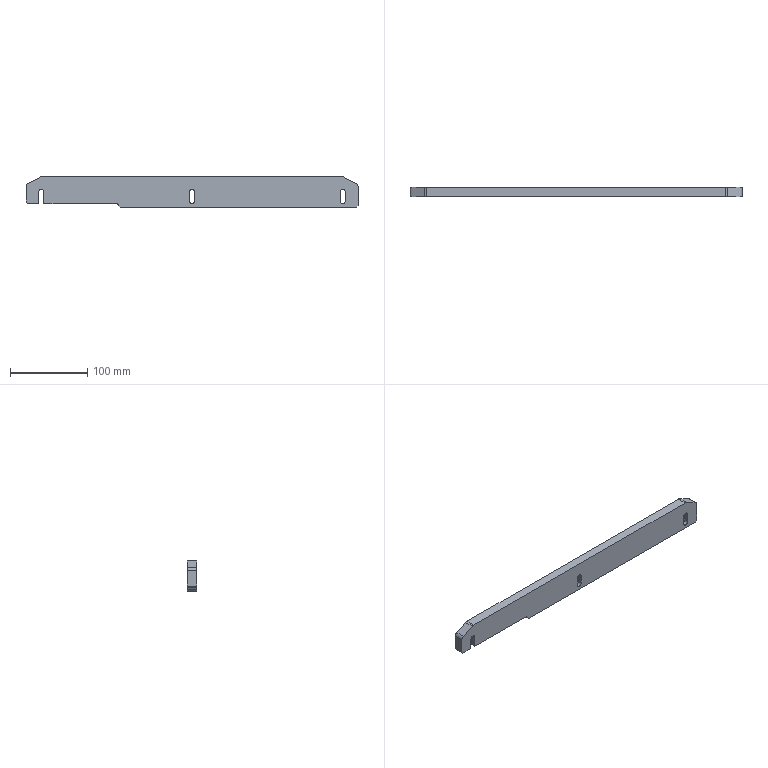Part | 1 solid | 43 faces | box 430.5 x 12 x 40 mm | volume 190634 mm3 | plane 28 | cylinder 15 | commonest cylinder face diameters 6.6 x5 11 x5 10 x4 6 x1
STEP:
#1=CARTESIAN_POINT('',(-95.25,-6.,-18.));
#2=VERTEX_POINT('',#1);
#3=CARTESIAN_POINT('',(-93.25,-6.,-20.));
#4=VERTEX_POINT('',#3);
#5=CARTESIAN_POINT('',(-93.25,-6.,-20.));
#6=DIRECTION('',(0.7071,0.,-0.7071));
#7=VECTOR('',#6,1000.);
#8=LINE('',#5,#7);
#9=EDGE_CURVE('',#2,#4,#8,.T.);
#10=ORIENTED_EDGE('',*,*,#9,.F.);
#11=CARTESIAN_POINT('',(-95.25,6.,-18.));
#12=VERTEX_POINT('',#11);
#13=CARTESIAN_POINT('',(-95.25,6.,-18.));
#14=DIRECTION('',(0.,1.,0.));
#15=VECTOR('',#14,1000.);
#16=LINE('',#13,#15);
#17=EDGE_CURVE('',#2,#12,#16,.T.);
#18=ORIENTED_EDGE('',*,*,#17,.T.);
#19=CARTESIAN_POINT('',(-93.25,6.,-20.));
#20=VERTEX_POINT('',#19);
#21=CARTESIAN_POINT('',(-56.625,6.,-56.625));
#22=DIRECTION('',(-0.7071,0.,0.7071));
#23=VECTOR('',#22,1000.);
#24=LINE('',#21,#23);
#25=EDGE_CURVE('',#20,#12,#24,.T.);
#26=ORIENTED_EDGE('',*,*,#25,.F.);
#27=CARTESIAN_POINT('',(-93.25,6.,-20.));
#28=DIRECTION('',(0.,1.,0.));
#29=VECTOR('',#28,1000.);
#30=LINE('',#27,#29);
#31=EDGE_CURVE('',#4,#20,#30,.T.);
#32=ORIENTED_EDGE('',*,*,#31,.F.);
#33=EDGE_LOOP('',(#10,#18,#26,#32));
#34=FACE_BOUND('',#33,.T.);
#35=CARTESIAN_POINT('',(-93.25,6.,-20.));
#36=DIRECTION('',(0.7071,0.,0.7071));
#37=DIRECTION('',(0.,1.,0.));
#38=AXIS2_PLACEMENT_3D('',#35,#36,#37);
#39=PLANE('',#38);
#40=ADVANCED_FACE('',(#34),#39,.F.);
#41=CARTESIAN_POINT('',(-215.25,-6.,-13.));
#42=VERTEX_POINT('',#41);
#43=CARTESIAN_POINT('',(-213.25,-6.,-15.));
#44=VERTEX_POINT('',#43);
#45=CARTESIAN_POINT('',(-213.25,-6.,-15.));
#46=DIRECTION('',(0.7071,0.,-0.7071));
#47=VECTOR('',#46,1000.);
#48=LINE('',#45,#47);
#49=EDGE_CURVE('',#42,#44,#48,.T.);
#50=ORIENTED_EDGE('',*,*,#49,.F.);
#51=CARTESIAN_POINT('',(-215.25,6.,-13.));
#52=VERTEX_POINT('',#51);
#53=CARTESIAN_POINT('',(-215.25,6.,-13.));
#54=DIRECTION('',(0.,-1.,0.));
#55=VECTOR('',#54,1000.);
#56=LINE('',#53,#55);
#57=EDGE_CURVE('',#52,#42,#56,.T.);
#58=ORIENTED_EDGE('',*,*,#57,.F.);
#59=CARTESIAN_POINT('',(-213.25,6.,-15.));
#60=VERTEX_POINT('',#59);
#61=CARTESIAN_POINT('',(-114.125,6.,-114.125));
#62=DIRECTION('',(-0.7071,0.,0.7071));
#63=VECTOR('',#62,1000.);
#64=LINE('',#61,#63);
#65=EDGE_CURVE('',#60,#52,#64,.T.);
#66=ORIENTED_EDGE('',*,*,#65,.F.);
#67=CARTESIAN_POINT('',(-213.25,-6.,-15.));
#68=DIRECTION('',(0.,1.,0.));
#69=VECTOR('',#68,1000.);
#70=LINE('',#67,#69);
#71=EDGE_CURVE('',#44,#60,#70,.T.);
#72=ORIENTED_EDGE('',*,*,#71,.F.);
#73=EDGE_LOOP('',(#50,#58,#66,#72));
#74=FACE_BOUND('',#73,.T.);
#75=CARTESIAN_POINT('',(-213.25,-6.,-15.));
#76=DIRECTION('',(0.7071,0.,0.7071));
#77=DIRECTION('',(0.,1.,0.));
#78=AXIS2_PLACEMENT_3D('',#75,#76,#77);
#79=PLANE('',#78);
#80=ADVANCED_FACE('',(#74),#79,.F.);
#81=CARTESIAN_POINT('',(-98.25,-6.,-15.));
#82=VERTEX_POINT('',#81);
#83=CARTESIAN_POINT('',(-98.25,-6.,-18.));
#84=DIRECTION('',(0.,1.,0.));
#85=DIRECTION('',(0.,0.,1.));
#86=AXIS2_PLACEMENT_3D('',#83,#84,#85);
#87=CIRCLE('',#86,3.);
#88=EDGE_CURVE('',#82,#2,#87,.T.);
#89=ORIENTED_EDGE('',*,*,#88,.F.);
#90=CARTESIAN_POINT('',(-98.25,6.,-15.));
#91=VERTEX_POINT('',#90);
#92=CARTESIAN_POINT('',(-98.25,-6.,-15.));
#93=DIRECTION('',(0.,-1.,0.));
#94=VECTOR('',#93,1000.);
#95=LINE('',#92,#94);
#96=EDGE_CURVE('',#91,#82,#95,.T.);
#97=ORIENTED_EDGE('',*,*,#96,.F.);
#98=CARTESIAN_POINT('',(-98.25,6.,-18.));
#99=DIRECTION('',(0.,-1.,0.));
#100=DIRECTION('',(0.,0.,1.));
#101=AXIS2_PLACEMENT_3D('',#98,#99,#100);
#102=CIRCLE('',#101,3.);
#103=EDGE_CURVE('',#12,#91,#102,.T.);
#104=ORIENTED_EDGE('',*,*,#103,.F.);
#105=ORIENTED_EDGE('',*,*,#17,.F.);
#106=EDGE_LOOP('',(#89,#97,#104,#105));
#107=FACE_BOUND('',#106,.T.);
#108=CARTESIAN_POINT('',(-98.25,-6.,-18.));
#109=DIRECTION('',(0.,-1.,0.));
#110=DIRECTION('',(0.,0.,-1.));
#111=AXIS2_PLACEMENT_3D('',#108,#109,#110);
#112=CYLINDRICAL_SURFACE('',#111,3.);
#113=ADVANCED_FACE('',(#107),#112,.F.);
#114=CARTESIAN_POINT('',(-191.95,-6.,-15.));
#115=VERTEX_POINT('',#114);
#116=CARTESIAN_POINT('',(-95.25,-6.,-15.));
#117=DIRECTION('',(1.,0.,0.));
#118=VECTOR('',#117,1000.);
#119=LINE('',#116,#118);
#120=EDGE_CURVE('',#115,#82,#119,.T.);
#121=ORIENTED_EDGE('',*,*,#120,.F.);
#122=CARTESIAN_POINT('',(-191.95,-0.8,-15.));
#123=VERTEX_POINT('',#122);
#124=CARTESIAN_POINT('',(-191.95,-6.,-15.));
#125=DIRECTION('',(0.,1.,0.));
#126=VECTOR('',#125,1000.);
#127=LINE('',#124,#126);
#128=EDGE_CURVE('',#115,#123,#127,.T.);
#129=ORIENTED_EDGE('',*,*,#128,.T.);
#130=CARTESIAN_POINT('',(-189.75,-0.8,-15.));
#131=VERTEX_POINT('',#130);
#132=CARTESIAN_POINT('',(198.55,-0.8,-15.));
#133=DIRECTION('',(-1.,0.,0.));
#134=VECTOR('',#133,1000.);
#135=LINE('',#132,#134);
#136=EDGE_CURVE('',#131,#123,#135,.T.);
#137=ORIENTED_EDGE('',*,*,#136,.F.);
#138=CARTESIAN_POINT('',(-189.75,6.,-15.));
#139=VERTEX_POINT('',#138);
#140=CARTESIAN_POINT('',(-189.75,-12.202,-15.));
#141=DIRECTION('',(0.,1.,0.));
#142=VECTOR('',#141,1000.);
#143=LINE('',#140,#142);
#144=EDGE_CURVE('',#131,#139,#143,.T.);
#145=ORIENTED_EDGE('',*,*,#144,.T.);
#146=CARTESIAN_POINT('',(-95.25,6.,-15.));
#147=DIRECTION('',(1.,0.,0.));
#148=VECTOR('',#147,1000.);
#149=LINE('',#146,#148);
#150=EDGE_CURVE('',#139,#91,#149,.T.);
#151=ORIENTED_EDGE('',*,*,#150,.T.);
#152=ORIENTED_EDGE('',*,*,#96,.T.);
#153=EDGE_LOOP('',(#121,#129,#137,#145,#151,#152));
#154=FACE_BOUND('',#153,.T.);
#155=CARTESIAN_POINT('',(-95.25,-6.,-15.));
#156=DIRECTION('',(0.,0.,1.));
#157=DIRECTION('',(1.,0.,0.));
#158=AXIS2_PLACEMENT_3D('',#155,#156,#157);
#159=PLANE('',#158);
#160=ADVANCED_FACE('',(#154),#159,.F.);
#161=CARTESIAN_POINT('',(-198.55,-0.8,-15.));
#162=VERTEX_POINT('',#161);
#163=CARTESIAN_POINT('',(-200.75,-0.8,-15.));
#164=VERTEX_POINT('',#163);
#165=CARTESIAN_POINT('',(198.55,-0.8,-15.));
#166=DIRECTION('',(-1.,0.,0.));
#167=VECTOR('',#166,1000.);
#168=LINE('',#165,#167);
#169=EDGE_CURVE('',#162,#164,#168,.T.);
#170=ORIENTED_EDGE('',*,*,#169,.F.);
#171=CARTESIAN_POINT('',(-198.55,-6.,-15.));
#172=VERTEX_POINT('',#171);
#173=CARTESIAN_POINT('',(-198.55,-6.,-15.));
#174=DIRECTION('',(0.,1.,0.));
#175=VECTOR('',#174,1000.);
#176=LINE('',#173,#175);
#177=EDGE_CURVE('',#172,#162,#176,.T.);
#178=ORIENTED_EDGE('',*,*,#177,.F.);
#179=CARTESIAN_POINT('',(-95.25,-6.,-15.));
#180=DIRECTION('',(1.,0.,0.));
#181=VECTOR('',#180,1000.);
#182=LINE('',#179,#181);
#183=EDGE_CURVE('',#44,#172,#182,.T.);
#184=ORIENTED_EDGE('',*,*,#183,.F.);
#185=ORIENTED_EDGE('',*,*,#71,.T.);
#186=CARTESIAN_POINT('',(-200.75,6.,-15.));
#187=VERTEX_POINT('',#186);
#188=CARTESIAN_POINT('',(-95.25,6.,-15.));
#189=DIRECTION('',(1.,0.,0.));
#190=VECTOR('',#189,1000.);
#191=LINE('',#188,#190);
#192=EDGE_CURVE('',#60,#187,#191,.T.);
#193=ORIENTED_EDGE('',*,*,#192,.T.);
#194=CARTESIAN_POINT('',(-200.75,-12.202,-15.));
#195=DIRECTION('',(0.,1.,0.));
#196=VECTOR('',#195,1000.);
#197=LINE('',#194,#196);
#198=EDGE_CURVE('',#164,#187,#197,.T.);
#199=ORIENTED_EDGE('',*,*,#198,.F.);
#200=EDGE_LOOP('',(#170,#178,#184,#185,#193,#199));
#201=FACE_BOUND('',#200,.T.);
#202=CARTESIAN_POINT('',(-95.25,-6.,-15.));
#203=DIRECTION('',(0.,0.,1.));
#204=DIRECTION('',(1.,0.,0.));
#205=AXIS2_PLACEMENT_3D('',#202,#203,#204);
#206=PLANE('',#205);
#207=ADVANCED_FACE('',(#201),#206,.F.);
#208=CARTESIAN_POINT('',(215.25,6.,-18.));
#209=VERTEX_POINT('',#208);
#210=CARTESIAN_POINT('',(213.25,6.,-20.));
#211=VERTEX_POINT('',#210);
#212=CARTESIAN_POINT('',(116.625,6.,-116.625));
#213=DIRECTION('',(-0.7071,0.,-0.7071));
#214=VECTOR('',#213,1000.);
#215=LINE('',#212,#214);
#216=EDGE_CURVE('',#209,#211,#215,.T.);
#217=ORIENTED_EDGE('',*,*,#216,.F.);
#218=CARTESIAN_POINT('',(215.25,-6.,-18.));
#219=VERTEX_POINT('',#218);
#220=CARTESIAN_POINT('',(215.25,6.,-18.));
#221=DIRECTION('',(0.,1.,0.));
#222=VECTOR('',#221,1000.);
#223=LINE('',#220,#222);
#224=EDGE_CURVE('',#219,#209,#223,.T.);
#225=ORIENTED_EDGE('',*,*,#224,.F.);
#226=CARTESIAN_POINT('',(213.25,-6.,-20.));
#227=VERTEX_POINT('',#226);
#228=CARTESIAN_POINT('',(213.25,-6.,-20.));
#229=DIRECTION('',(0.7071,0.,0.7071));
#230=VECTOR('',#229,1000.);
#231=LINE('',#228,#230);
#232=EDGE_CURVE('',#227,#219,#231,.T.);
#233=ORIENTED_EDGE('',*,*,#232,.F.);
#234=CARTESIAN_POINT('',(213.25,6.,-20.));
#235=DIRECTION('',(0.,-1.,0.));
#236=VECTOR('',#235,1000.);
#237=LINE('',#234,#236);
#238=EDGE_CURVE('',#211,#227,#237,.T.);
#239=ORIENTED_EDGE('',*,*,#238,.F.);
#240=EDGE_LOOP('',(#217,#225,#233,#239));
#241=FACE_BOUND('',#240,.T.);
#242=CARTESIAN_POINT('',(213.25,6.,-20.));
#243=DIRECTION('',(-0.7071,0.,0.7071));
#244=DIRECTION('',(0.,-1.,0.));
#245=AXIS2_PLACEMENT_3D('',#242,#243,#244);
#246=PLANE('',#245);
#247=ADVANCED_FACE('',(#241),#246,.F.);
#248=CARTESIAN_POINT('',(-194.07,-6.,20.));
#249=VERTEX_POINT('',#248);
#250=CARTESIAN_POINT('',(-196.306,-6.,19.472));
#251=VERTEX_POINT('',#250);
#252=CARTESIAN_POINT('',(-194.07,-6.,15.));
#253=DIRECTION('',(0.,-1.,0.));
#254=DIRECTION('',(0.,0.,1.));
#255=AXIS2_PLACEMENT_3D('',#252,#253,#254);
#256=CIRCLE('',#255,5.);
#257=EDGE_CURVE('',#249,#251,#256,.T.);
#258=ORIENTED_EDGE('',*,*,#257,.F.);
#259=CARTESIAN_POINT('',(-194.07,6.,20.));
#260=VERTEX_POINT('',#259);
#261=CARTESIAN_POINT('',(-194.07,-6.,20.));
#262=DIRECTION('',(0.,-1.,0.));
#263=VECTOR('',#262,1000.);
#264=LINE('',#261,#263);
#265=EDGE_CURVE('',#260,#249,#264,.T.);
#266=ORIENTED_EDGE('',*,*,#265,.F.);
#267=CARTESIAN_POINT('',(-196.306,6.,19.472));
#268=VERTEX_POINT('',#267);
#269=CARTESIAN_POINT('',(-194.07,6.,15.));
#270=DIRECTION('',(0.,1.,0.));
#271=DIRECTION('',(0.,0.,1.));
#272=AXIS2_PLACEMENT_3D('',#269,#270,#271);
#273=CIRCLE('',#272,5.);
#274=EDGE_CURVE('',#268,#260,#273,.T.);
#275=ORIENTED_EDGE('',*,*,#274,.F.);
#276=CARTESIAN_POINT('',(-196.306,6.,19.472));
#277=DIRECTION('',(0.,1.,0.));
#278=VECTOR('',#277,1000.);
#279=LINE('',#276,#278);
#280=EDGE_CURVE('',#251,#268,#279,.T.);
#281=ORIENTED_EDGE('',*,*,#280,.F.);
#282=EDGE_LOOP('',(#258,#266,#275,#281));
#283=FACE_BOUND('',#282,.T.);
#284=CARTESIAN_POINT('',(-194.07,-6.,15.));
#285=DIRECTION('',(0.,-1.,0.));
#286=DIRECTION('',(0.,0.,-1.));
#287=AXIS2_PLACEMENT_3D('',#284,#285,#286);
#288=CYLINDRICAL_SURFACE('',#287,5.);
#289=ADVANCED_FACE('',(#283),#288,.T.);
#290=CARTESIAN_POINT('',(-212.486,-6.,11.382));
#291=VERTEX_POINT('',#290);
#292=CARTESIAN_POINT('',(-215.25,-6.,6.91));
#293=VERTEX_POINT('',#292);
#294=CARTESIAN_POINT('',(-210.25,-6.,6.91));
#295=DIRECTION('',(0.,-1.,0.));
#296=DIRECTION('',(0.,0.,1.));
#297=AXIS2_PLACEMENT_3D('',#294,#295,#296);
#298=CIRCLE('',#297,5.);
#299=EDGE_CURVE('',#291,#293,#298,.T.);
#300=ORIENTED_EDGE('',*,*,#299,.F.);
#301=CARTESIAN_POINT('',(-212.486,6.,11.382));
#302=VERTEX_POINT('',#301);
#303=CARTESIAN_POINT('',(-212.486,-6.,11.382));
#304=DIRECTION('',(0.,-1.,0.));
#305=VECTOR('',#304,1000.);
#306=LINE('',#303,#305);
#307=EDGE_CURVE('',#302,#291,#306,.T.);
#308=ORIENTED_EDGE('',*,*,#307,.F.);
#309=CARTESIAN_POINT('',(-215.25,6.,6.91));
#310=VERTEX_POINT('',#309);
#311=CARTESIAN_POINT('',(-210.25,6.,6.91));
#312=DIRECTION('',(0.,1.,0.));
#313=DIRECTION('',(0.,0.,1.));
#314=AXIS2_PLACEMENT_3D('',#311,#312,#313);
#315=CIRCLE('',#314,5.);
#316=EDGE_CURVE('',#310,#302,#315,.T.);
#317=ORIENTED_EDGE('',*,*,#316,.F.);
#318=CARTESIAN_POINT('',(-215.25,6.,6.91));
#319=DIRECTION('',(0.,1.,0.));
#320=VECTOR('',#319,1000.);
#321=LINE('',#318,#320);
#322=EDGE_CURVE('',#293,#310,#321,.T.);
#323=ORIENTED_EDGE('',*,*,#322,.F.);
#324=EDGE_LOOP('',(#300,#308,#317,#323));
#325=FACE_BOUND('',#324,.T.);
#326=CARTESIAN_POINT('',(-210.25,6.,6.91));
#327=DIRECTION('',(0.,-1.,0.));
#328=DIRECTION('',(0.,0.,-1.));
#329=AXIS2_PLACEMENT_3D('',#326,#327,#328);
#330=CYLINDRICAL_SURFACE('',#329,5.);
#331=ADVANCED_FACE('',(#325),#330,.T.);
#332=CARTESIAN_POINT('',(196.306,-6.,19.472));
#333=VERTEX_POINT('',#332);
#334=CARTESIAN_POINT('',(194.07,-6.,20.));
#335=VERTEX_POINT('',#334);
#336=CARTESIAN_POINT('',(194.07,-6.,15.));
#337=DIRECTION('',(0.,-1.,0.));
#338=DIRECTION('',(0.,0.,1.));
#339=AXIS2_PLACEMENT_3D('',#336,#337,#338);
#340=CIRCLE('',#339,5.);
#341=EDGE_CURVE('',#333,#335,#340,.T.);
#342=ORIENTED_EDGE('',*,*,#341,.F.);
#343=CARTESIAN_POINT('',(196.306,6.,19.472));
#344=VERTEX_POINT('',#343);
#345=CARTESIAN_POINT('',(196.306,-6.,19.472));
#346=DIRECTION('',(0.,-1.,0.));
#347=VECTOR('',#346,1000.);
#348=LINE('',#345,#347);
#349=EDGE_CURVE('',#344,#333,#348,.T.);
#350=ORIENTED_EDGE('',*,*,#349,.F.);
#351=CARTESIAN_POINT('',(194.07,6.,20.));
#352=VERTEX_POINT('',#351);
#353=CARTESIAN_POINT('',(194.07,6.,15.));
#354=DIRECTION('',(0.,1.,0.));
#355=DIRECTION('',(0.,0.,1.));
#356=AXIS2_PLACEMENT_3D('',#353,#354,#355);
#357=CIRCLE('',#356,5.);
#358=EDGE_CURVE('',#352,#344,#357,.T.);
#359=ORIENTED_EDGE('',*,*,#358,.F.);
#360=CARTESIAN_POINT('',(194.07,6.,20.));
#361=DIRECTION('',(0.,1.,0.));
#362=VECTOR('',#361,1000.);
#363=LINE('',#360,#362);
#364=EDGE_CURVE('',#335,#352,#363,.T.);
#365=ORIENTED_EDGE('',*,*,#364,.F.);
#366=EDGE_LOOP('',(#342,#350,#359,#365));
#367=FACE_BOUND('',#366,.T.);
#368=CARTESIAN_POINT('',(194.07,6.,15.));
#369=DIRECTION('',(0.,1.,0.));
#370=DIRECTION('',(0.,0.,1.));
#371=AXIS2_PLACEMENT_3D('',#368,#369,#370);
#372=CYLINDRICAL_SURFACE('',#371,5.);
#373=ADVANCED_FACE('',(#367),#372,.T.);
#374=CARTESIAN_POINT('',(215.25,-6.,6.91));
#375=VERTEX_POINT('',#374);
#376=CARTESIAN_POINT('',(212.486,-6.,11.382));
#377=VERTEX_POINT('',#376);
#378=CARTESIAN_POINT('',(210.25,-6.,6.91));
#379=DIRECTION('',(0.,-1.,0.));
#380=DIRECTION('',(0.,0.,1.));
#381=AXIS2_PLACEMENT_3D('',#378,#379,#380);
#382=CIRCLE('',#381,5.);
#383=EDGE_CURVE('',#375,#377,#382,.T.);
#384=ORIENTED_EDGE('',*,*,#383,.F.);
#385=CARTESIAN_POINT('',(215.25,6.,6.91));
#386=VERTEX_POINT('',#385);
#387=CARTESIAN_POINT('',(215.25,6.,6.91));
#388=DIRECTION('',(0.,-1.,0.));
#389=VECTOR('',#388,1000.);
#390=LINE('',#387,#389);
#391=EDGE_CURVE('',#386,#375,#390,.T.);
#392=ORIENTED_EDGE('',*,*,#391,.F.);
#393=CARTESIAN_POINT('',(212.486,6.,11.382));
#394=VERTEX_POINT('',#393);
#395=CARTESIAN_POINT('',(210.25,6.,6.91));
#396=DIRECTION('',(0.,1.,0.));
#397=DIRECTION('',(0.,0.,1.));
#398=AXIS2_PLACEMENT_3D('',#395,#396,#397);
#399=CIRCLE('',#398,5.);
#400=EDGE_CURVE('',#394,#386,#399,.T.);
#401=ORIENTED_EDGE('',*,*,#400,.F.);
#402=CARTESIAN_POINT('',(212.486,-6.,11.382));
#403=DIRECTION('',(0.,1.,0.));
#404=VECTOR('',#403,1000.);
#405=LINE('',#402,#404);
#406=EDGE_CURVE('',#377,#394,#405,.T.);
#407=ORIENTED_EDGE('',*,*,#406,.F.);
#408=EDGE_LOOP('',(#384,#392,#401,#407));
#409=FACE_BOUND('',#408,.T.);
#410=CARTESIAN_POINT('',(210.25,-6.,6.91));
#411=DIRECTION('',(0.,1.,0.));
#412=DIRECTION('',(0.,0.,1.));
#413=AXIS2_PLACEMENT_3D('',#410,#411,#412);
#414=CYLINDRICAL_SURFACE('',#413,5.);
#415=ADVANCED_FACE('',(#409),#414,.T.);
#416=CARTESIAN_POINT('',(200.75,6.,-12.));
#417=VERTEX_POINT('',#416);
#418=CARTESIAN_POINT('',(200.75,-0.8,-12.));
#419=VERTEX_POINT('',#418);
#420=CARTESIAN_POINT('',(200.75,-0.8,-12.));
#421=DIRECTION('',(0.,-1.,0.));
#422=VECTOR('',#421,1000.);
#423=LINE('',#420,#422);
#424=EDGE_CURVE('',#417,#419,#423,.T.);
#425=ORIENTED_EDGE('',*,*,#424,.T.);
#426=CARTESIAN_POINT('',(200.75,-0.8,0.));
#427=VERTEX_POINT('',#426);
#428=CARTESIAN_POINT('',(200.75,-0.8,0.));
#429=DIRECTION('',(0.,0.,-1.));
#430=VECTOR('',#429,1000.);
#431=LINE('',#428,#430);
#432=EDGE_CURVE('',#427,#419,#431,.T.);
#433=ORIENTED_EDGE('',*,*,#432,.F.);
#434=CARTESIAN_POINT('',(200.75,6.,0.));
#435=VERTEX_POINT('',#434);
#436=CARTESIAN_POINT('',(200.75,-0.8,0.));
#437=DIRECTION('',(0.,-1.,0.));
#438=VECTOR('',#437,1000.);
#439=LINE('',#436,#438);
#440=EDGE_CURVE('',#435,#427,#439,.T.);
#441=ORIENTED_EDGE('',*,*,#440,.F.);
#442=CARTESIAN_POINT('',(200.75,6.,0.));
#443=DIRECTION('',(0.,0.,-1.));
#444=VECTOR('',#443,1000.);
#445=LINE('',#442,#444);
#446=EDGE_CURVE('',#435,#417,#445,.T.);
#447=ORIENTED_EDGE('',*,*,#446,.T.);
#448=EDGE_LOOP('',(#425,#433,#441,#447));
#449=FACE_BOUND('',#448,.T.);
#450=CARTESIAN_POINT('',(200.75,-0.8,0.));
#451=DIRECTION('',(1.,0.,0.));
#452=DIRECTION('',(0.,1.,0.));
#453=AXIS2_PLACEMENT_3D('',#450,#451,#452);
#454=PLANE('',#453);
#455=ADVANCED_FACE('',(#449),#454,.F.);
#456=CARTESIAN_POINT('',(198.55,-0.8,-12.));
#457=VERTEX_POINT('',#456);
#458=CARTESIAN_POINT('',(198.55,-6.,-12.));
#459=VERTEX_POINT('',#458);
#460=CARTESIAN_POINT('',(198.55,-6.,-12.));
#461=DIRECTION('',(0.,-1.,0.));
#462=VECTOR('',#461,1000.);
#463=LINE('',#460,#462);
#464=EDGE_CURVE('',#457,#459,#463,.T.);
#465=ORIENTED_EDGE('',*,*,#464,.T.);
#466=CARTESIAN_POINT('',(198.55,-6.,0.));
#467=VERTEX_POINT('',#466);
#468=CARTESIAN_POINT('',(198.55,-6.,0.));
#469=DIRECTION('',(0.,0.,-1.));
#470=VECTOR('',#469,1000.);
#471=LINE('',#468,#470);
#472=EDGE_CURVE('',#467,#459,#471,.T.);
#473=ORIENTED_EDGE('',*,*,#472,.F.);
#474=CARTESIAN_POINT('',(198.55,-0.8,0.));
#475=VERTEX_POINT('',#474);
#476=CARTESIAN_POINT('',(198.55,-6.,0.));
#477=DIRECTION('',(0.,-1.,0.));
#478=VECTOR('',#477,1000.);
#479=LINE('',#476,#478);
#480=EDGE_CURVE('',#475,#467,#479,.T.);
#481=ORIENTED_EDGE('',*,*,#480,.F.);
#482=CARTESIAN_POINT('',(198.55,-0.8,0.));
#483=DIRECTION('',(0.,0.,-1.));
#484=VECTOR('',#483,1000.);
#485=LINE('',#482,#484);
#486=EDGE_CURVE('',#475,#457,#485,.T.);
#487=ORIENTED_EDGE('',*,*,#486,.T.);
#488=EDGE_LOOP('',(#465,#473,#481,#487));
#489=FACE_BOUND('',#488,.T.);
#490=CARTESIAN_POINT('',(198.55,-6.,0.));
#491=DIRECTION('',(1.,0.,0.));
#492=DIRECTION('',(0.,1.,0.));
#493=AXIS2_PLACEMENT_3D('',#490,#491,#492);
#494=PLANE('',#493);
#495=ADVANCED_FACE('',(#489),#494,.F.);
#496=CARTESIAN_POINT('',(191.95,-6.,-12.));
#497=VERTEX_POINT('',#496);
#498=CARTESIAN_POINT('',(191.95,-0.8,-12.));
#499=VERTEX_POINT('',#498);
#500=CARTESIAN_POINT('',(191.95,6.,-12.));
#501=DIRECTION('',(0.,1.,0.));
#502=VECTOR('',#501,1000.);
#503=LINE('',#500,#502);
#504=EDGE_CURVE('',#497,#499,#503,.T.);
#505=ORIENTED_EDGE('',*,*,#504,.T.);
#506=CARTESIAN_POINT('',(191.95,-0.8,0.));
#507=VERTEX_POINT('',#506);
#508=CARTESIAN_POINT('',(191.95,-0.8,0.));
#509=DIRECTION('',(0.,0.,-1.));
#510=VECTOR('',#509,1000.);
#511=LINE('',#508,#510);
#512=EDGE_CURVE('',#507,#499,#511,.T.);
#513=ORIENTED_EDGE('',*,*,#512,.F.);
#514=CARTESIAN_POINT('',(191.95,-6.,0.));
#515=VERTEX_POINT('',#514);
#516=CARTESIAN_POINT('',(191.95,6.,0.));
#517=DIRECTION('',(0.,-1.,0.));
#518=VECTOR('',#517,1000.);
#519=LINE('',#516,#518);
#520=EDGE_CURVE('',#507,#515,#519,.T.);
#521=ORIENTED_EDGE('',*,*,#520,.T.);
#522=CARTESIAN_POINT('',(191.95,-6.,0.));
#523=DIRECTION('',(0.,0.,-1.));
#524=VECTOR('',#523,1000.);
#525=LINE('',#522,#524);
#526=EDGE_CURVE('',#515,#497,#525,.T.);
#527=ORIENTED_EDGE('',*,*,#526,.T.);
#528=EDGE_LOOP('',(#505,#513,#521,#527));
#529=FACE_BOUND('',#528,.T.);
#530=CARTESIAN_POINT('',(191.95,6.,0.));
#531=DIRECTION('',(-1.,0.,0.));
#532=DIRECTION('',(0.,0.,1.));
#533=AXIS2_PLACEMENT_3D('',#530,#531,#532);
#534=PLANE('',#533);
#535=ADVANCED_FACE('',(#529),#534,.F.);
#536=CARTESIAN_POINT('',(189.75,-0.8,-12.));
#537=VERTEX_POINT('',#536);
#538=CARTESIAN_POINT('',(189.75,6.,-12.));
#539=VERTEX_POINT('',#538);
#540=CARTESIAN_POINT('',(189.75,6.,-12.));
#541=DIRECTION('',(0.,1.,0.));
#542=VECTOR('',#541,1000.);
#543=LINE('',#540,#542);
#544=EDGE_CURVE('',#537,#539,#543,.T.);
#545=ORIENTED_EDGE('',*,*,#544,.T.);
#546=CARTESIAN_POINT('',(189.75,6.,0.));
#547=VERTEX_POINT('',#546);
#548=CARTESIAN_POINT('',(189.75,6.,0.));
#549=DIRECTION('',(0.,0.,-1.));
#550=VECTOR('',#549,1000.);
#551=LINE('',#548,#550);
#552=EDGE_CURVE('',#547,#539,#551,.T.);
#553=ORIENTED_EDGE('',*,*,#552,.F.);
#554=CARTESIAN_POINT('',(189.75,-0.8,0.));
#555=VERTEX_POINT('',#554);
#556=CARTESIAN_POINT('',(189.75,6.,0.));
#557=DIRECTION('',(0.,-1.,0.));
#558=VECTOR('',#557,1000.);
#559=LINE('',#556,#558);
#560=EDGE_CURVE('',#547,#555,#559,.T.);
#561=ORIENTED_EDGE('',*,*,#560,.T.);
#562=CARTESIAN_POINT('',(189.75,-0.8,0.));
#563=DIRECTION('',(0.,0.,-1.));
#564=VECTOR('',#563,1000.);
#565=LINE('',#562,#564);
#566=EDGE_CURVE('',#555,#537,#565,.T.);
#567=ORIENTED_EDGE('',*,*,#566,.T.);
#568=EDGE_LOOP('',(#545,#553,#561,#567));
#569=FACE_BOUND('',#568,.T.);
#570=CARTESIAN_POINT('',(189.75,6.,0.));
#571=DIRECTION('',(-1.,0.,0.));
#572=DIRECTION('',(0.,0.,1.));
#573=AXIS2_PLACEMENT_3D('',#570,#571,#572);
#574=PLANE('',#573);
#575=ADVANCED_FACE('',(#569),#574,.F.);
#576=CARTESIAN_POINT('',(195.25,-0.8,-12.));
#577=DIRECTION('',(0.,1.,0.));
#578=DIRECTION('',(0.,0.,1.));
#579=AXIS2_PLACEMENT_3D('',#576,#577,#578);
#580=CIRCLE('',#579,5.5);
#581=EDGE_CURVE('',#419,#537,#580,.T.);
#582=ORIENTED_EDGE('',*,*,#581,.F.);
#583=ORIENTED_EDGE('',*,*,#424,.F.);
#584=CARTESIAN_POINT('',(195.25,6.,-12.));
#585=DIRECTION('',(0.,1.,0.));
#586=DIRECTION('',(0.,0.,1.));
#587=AXIS2_PLACEMENT_3D('',#584,#585,#586);
#588=CIRCLE('',#587,5.5);
#589=EDGE_CURVE('',#417,#539,#588,.T.);
#590=ORIENTED_EDGE('',*,*,#589,.T.);
#591=ORIENTED_EDGE('',*,*,#544,.F.);
#592=EDGE_LOOP('',(#582,#583,#590,#591));
#593=FACE_BOUND('',#592,.T.);
#594=CARTESIAN_POINT('',(195.25,6.,-12.));
#595=DIRECTION('',(0.,1.,0.));
#596=DIRECTION('',(0.,0.,1.));
#597=AXIS2_PLACEMENT_3D('',#594,#595,#596);
#598=CYLINDRICAL_SURFACE('',#597,5.5);
#599=ADVANCED_FACE('',(#593),#598,.F.);
#600=CARTESIAN_POINT('',(195.25,-0.8,-12.));
#601=DIRECTION('',(0.,1.,0.));
#602=DIRECTION('',(0.,0.,1.));
#603=AXIS2_PLACEMENT_3D('',#600,#601,#602);
#604=CIRCLE('',#603,3.3);
#605=EDGE_CURVE('',#457,#499,#604,.T.);
#606=ORIENTED_EDGE('',*,*,#605,.F.);
#607=ORIENTED_EDGE('',*,*,#486,.F.);
#608=CARTESIAN_POINT('',(195.25,-0.8,0.));
#609=DIRECTION('',(0.,1.,0.));
#610=DIRECTION('',(0.,0.,1.));
#611=AXIS2_PLACEMENT_3D('',#608,#609,#610);
#612=CIRCLE('',#611,3.3);
#613=EDGE_CURVE('',#507,#475,#612,.T.);
#614=ORIENTED_EDGE('',*,*,#613,.F.);
#615=ORIENTED_EDGE('',*,*,#512,.T.);
#616=EDGE_LOOP('',(#606,#607,#614,#615));
#617=FACE_BOUND('',#616,.T.);
#618=ORIENTED_EDGE('',*,*,#566,.F.);
#619=CARTESIAN_POINT('',(195.25,-0.8,0.));
#620=DIRECTION('',(0.,1.,0.));
#621=DIRECTION('',(0.,0.,1.));
#622=AXIS2_PLACEMENT_3D('',#619,#620,#621);
#623=CIRCLE('',#622,5.5);
#624=EDGE_CURVE('',#555,#427,#623,.T.);
#625=ORIENTED_EDGE('',*,*,#624,.T.);
#626=ORIENTED_EDGE('',*,*,#432,.T.);
#627=ORIENTED_EDGE('',*,*,#581,.T.);
#628=EDGE_LOOP('',(#618,#625,#626,#627));
#629=FACE_BOUND('',#628,.T.);
#630=CARTESIAN_POINT('',(198.55,-0.8,-12.));
#631=DIRECTION('',(0.,-1.,0.));
#632=DIRECTION('',(0.,0.,-1.));
#633=AXIS2_PLACEMENT_3D('',#630,#631,#632);
#634=PLANE('',#633);
#635=ADVANCED_FACE('',(#617,#629),#634,.F.);
#636=CARTESIAN_POINT('',(195.25,-6.,-12.));
#637=DIRECTION('',(0.,1.,0.));
#638=DIRECTION('',(0.,0.,1.));
#639=AXIS2_PLACEMENT_3D('',#636,#637,#638);
#640=CIRCLE('',#639,3.3);
#641=EDGE_CURVE('',#459,#497,#640,.T.);
#642=ORIENTED_EDGE('',*,*,#641,.F.);
#643=ORIENTED_EDGE('',*,*,#464,.F.);
#644=ORIENTED_EDGE('',*,*,#605,.T.);
#645=ORIENTED_EDGE('',*,*,#504,.F.);
#646=EDGE_LOOP('',(#642,#643,#644,#645));
#647=FACE_BOUND('',#646,.T.);
#648=CARTESIAN_POINT('',(195.25,6.,-12.));
#649=DIRECTION('',(0.,1.,0.));
#650=DIRECTION('',(0.,0.,1.));
#651=AXIS2_PLACEMENT_3D('',#648,#649,#650);
#652=CYLINDRICAL_SURFACE('',#651,3.3);
#653=ADVANCED_FACE('',(#647),#652,.F.);
#654=CARTESIAN_POINT('',(-189.75,6.,0.));
#655=VERTEX_POINT('',#654);
#656=CARTESIAN_POINT('',(-189.75,6.,0.));
#657=DIRECTION('',(0.,0.,-1.));
#658=VECTOR('',#657,1000.);
#659=LINE('',#656,#658);
#660=EDGE_CURVE('',#655,#139,#659,.T.);
#661=ORIENTED_EDGE('',*,*,#660,.T.);
#662=ORIENTED_EDGE('',*,*,#144,.F.);
#663=CARTESIAN_POINT('',(-189.75,-0.8,0.));
#664=VERTEX_POINT('',#663);
#665=CARTESIAN_POINT('',(-189.75,-0.8,-12.));
#666=DIRECTION('',(0.,0.,-1.));
#667=VECTOR('',#666,1000.);
#668=LINE('',#665,#667);
#669=EDGE_CURVE('',#664,#131,#668,.T.);
#670=ORIENTED_EDGE('',*,*,#669,.F.);
#671=CARTESIAN_POINT('',(-189.75,-0.8,0.));
#672=DIRECTION('',(0.,-1.,0.));
#673=VECTOR('',#672,1000.);
#674=LINE('',#671,#673);
#675=EDGE_CURVE('',#655,#664,#674,.T.);
#676=ORIENTED_EDGE('',*,*,#675,.F.);
#677=EDGE_LOOP('',(#661,#662,#670,#676));
#678=FACE_BOUND('',#677,.T.);
#679=CARTESIAN_POINT('',(-189.75,-0.8,0.));
#680=DIRECTION('',(1.,0.,0.));
#681=DIRECTION('',(0.,1.,0.));
#682=AXIS2_PLACEMENT_3D('',#679,#680,#681);
#683=PLANE('',#682);
#684=ADVANCED_FACE('',(#678),#683,.F.);
#685=CARTESIAN_POINT('',(-191.95,-0.8,0.));
#686=VERTEX_POINT('',#685);
#687=CARTESIAN_POINT('',(-191.95,-0.8,0.));
#688=DIRECTION('',(0.,0.,-1.));
#689=VECTOR('',#688,1000.);
#690=LINE('',#687,#689);
#691=EDGE_CURVE('',#686,#123,#690,.T.);
#692=ORIENTED_EDGE('',*,*,#691,.T.);
#693=ORIENTED_EDGE('',*,*,#128,.F.);
#694=CARTESIAN_POINT('',(-191.95,-6.,0.));
#695=VERTEX_POINT('',#694);
#696=CARTESIAN_POINT('',(-191.95,-6.,0.));
#697=DIRECTION('',(0.,0.,-1.));
#698=VECTOR('',#697,1000.);
#699=LINE('',#696,#698);
#700=EDGE_CURVE('',#695,#115,#699,.T.);
#701=ORIENTED_EDGE('',*,*,#700,.F.);
#702=CARTESIAN_POINT('',(-191.95,-6.,0.));
#703=DIRECTION('',(0.,-1.,0.));
#704=VECTOR('',#703,1000.);
#705=LINE('',#702,#704);
#706=EDGE_CURVE('',#686,#695,#705,.T.);
#707=ORIENTED_EDGE('',*,*,#706,.F.);
#708=EDGE_LOOP('',(#692,#693,#701,#707));
#709=FACE_BOUND('',#708,.T.);
#710=CARTESIAN_POINT('',(-191.95,-6.,0.));
#711=DIRECTION('',(1.,0.,0.));
#712=DIRECTION('',(0.,1.,0.));
#713=AXIS2_PLACEMENT_3D('',#710,#711,#712);
#714=PLANE('',#713);
#715=ADVANCED_FACE('',(#709),#714,.F.);
#716=CARTESIAN_POINT('',(-198.55,-6.,0.));
#717=VERTEX_POINT('',#716);
#718=CARTESIAN_POINT('',(-198.55,-6.,0.));
#719=DIRECTION('',(0.,0.,-1.));
#720=VECTOR('',#719,1000.);
#721=LINE('',#718,#720);
#722=EDGE_CURVE('',#717,#172,#721,.T.);
#723=ORIENTED_EDGE('',*,*,#722,.T.);
#724=ORIENTED_EDGE('',*,*,#177,.T.);
#725=CARTESIAN_POINT('',(-198.55,-0.8,0.));
#726=VERTEX_POINT('',#725);
#727=CARTESIAN_POINT('',(-198.55,-0.8,-12.));
#728=DIRECTION('',(0.,0.,-1.));
#729=VECTOR('',#728,1000.);
#730=LINE('',#727,#729);
#731=EDGE_CURVE('',#726,#162,#730,.T.);
#732=ORIENTED_EDGE('',*,*,#731,.F.);
#733=CARTESIAN_POINT('',(-198.55,6.,0.));
#734=DIRECTION('',(0.,-1.,0.));
#735=VECTOR('',#734,1000.);
#736=LINE('',#733,#735);
#737=EDGE_CURVE('',#726,#717,#736,.T.);
#738=ORIENTED_EDGE('',*,*,#737,.T.);
#739=EDGE_LOOP('',(#723,#724,#732,#738));
#740=FACE_BOUND('',#739,.T.);
#741=CARTESIAN_POINT('',(-198.55,6.,0.));
#742=DIRECTION('',(-1.,0.,0.));
#743=DIRECTION('',(0.,0.,1.));
#744=AXIS2_PLACEMENT_3D('',#741,#742,#743);
#745=PLANE('',#744);
#746=ADVANCED_FACE('',(#740),#745,.F.);
#747=CARTESIAN_POINT('',(-200.75,-0.8,0.));
#748=VERTEX_POINT('',#747);
#749=CARTESIAN_POINT('',(-200.75,-0.8,0.));
#750=DIRECTION('',(0.,0.,-1.));
#751=VECTOR('',#750,1000.);
#752=LINE('',#749,#751);
#753=EDGE_CURVE('',#748,#164,#752,.T.);
#754=ORIENTED_EDGE('',*,*,#753,.T.);
#755=ORIENTED_EDGE('',*,*,#198,.T.);
#756=CARTESIAN_POINT('',(-200.75,6.,0.));
#757=VERTEX_POINT('',#756);
#758=CARTESIAN_POINT('',(-200.75,6.,0.));
#759=DIRECTION('',(0.,0.,-1.));
#760=VECTOR('',#759,1000.);
#761=LINE('',#758,#760);
#762=EDGE_CURVE('',#757,#187,#761,.T.);
#763=ORIENTED_EDGE('',*,*,#762,.F.);
#764=CARTESIAN_POINT('',(-200.75,6.,0.));
#765=DIRECTION('',(0.,-1.,0.));
#766=VECTOR('',#765,1000.);
#767=LINE('',#764,#766);
#768=EDGE_CURVE('',#757,#748,#767,.T.);
#769=ORIENTED_EDGE('',*,*,#768,.T.);
#770=EDGE_LOOP('',(#754,#755,#763,#769));
#771=FACE_BOUND('',#770,.T.);
#772=CARTESIAN_POINT('',(-200.75,6.,0.));
#773=DIRECTION('',(-1.,0.,0.));
#774=DIRECTION('',(0.,0.,1.));
#775=AXIS2_PLACEMENT_3D('',#772,#773,#774);
#776=PLANE('',#775);
#777=ADVANCED_FACE('',(#771),#776,.F.);
#778=ORIENTED_EDGE('',*,*,#136,.T.);
#779=ORIENTED_EDGE('',*,*,#691,.F.);
#780=CARTESIAN_POINT('',(-195.25,-0.8,0.));
#781=DIRECTION('',(0.,1.,0.));
#782=DIRECTION('',(0.,0.,-1.));
#783=AXIS2_PLACEMENT_3D('',#780,#781,#782);
#784=CIRCLE('',#783,3.3);
#785=EDGE_CURVE('',#726,#686,#784,.T.);
#786=ORIENTED_EDGE('',*,*,#785,.F.);
#787=ORIENTED_EDGE('',*,*,#731,.T.);
#788=ORIENTED_EDGE('',*,*,#169,.T.);
#789=ORIENTED_EDGE('',*,*,#753,.F.);
#790=CARTESIAN_POINT('',(-195.25,-0.8,0.));
#791=DIRECTION('',(0.,1.,0.));
#792=DIRECTION('',(0.,0.,-1.));
#793=AXIS2_PLACEMENT_3D('',#790,#791,#792);
#794=CIRCLE('',#793,5.5);
#795=EDGE_CURVE('',#748,#664,#794,.T.);
#796=ORIENTED_EDGE('',*,*,#795,.T.);
#797=ORIENTED_EDGE('',*,*,#669,.T.);
#798=EDGE_LOOP('',(#778,#779,#786,#787,#788,#789,#796,#797));
#799=FACE_BOUND('',#798,.T.);
#800=CARTESIAN_POINT('',(198.55,-0.8,-12.));
#801=DIRECTION('',(0.,-1.,0.));
#802=DIRECTION('',(0.,0.,-1.));
#803=AXIS2_PLACEMENT_3D('',#800,#801,#802);
#804=PLANE('',#803);
#805=ADVANCED_FACE('',(#799),#804,.F.);
#806=CARTESIAN_POINT('',(5.5,6.,-12.));
#807=VERTEX_POINT('',#806);
#808=CARTESIAN_POINT('',(5.5,-0.8,-12.));
#809=VERTEX_POINT('',#808);
#810=CARTESIAN_POINT('',(5.5,-0.8,-12.));
#811=DIRECTION('',(0.,-1.,0.));
#812=VECTOR('',#811,1000.);
#813=LINE('',#810,#812);
#814=EDGE_CURVE('',#807,#809,#813,.T.);
#815=ORIENTED_EDGE('',*,*,#814,.T.);
#816=CARTESIAN_POINT('',(5.5,-0.8,0.));
#817=VERTEX_POINT('',#816);
#818=CARTESIAN_POINT('',(5.5,-0.8,-12.));
#819=DIRECTION('',(0.,0.,-1.));
#820=VECTOR('',#819,1000.);
#821=LINE('',#818,#820);
#822=EDGE_CURVE('',#817,#809,#821,.T.);
#823=ORIENTED_EDGE('',*,*,#822,.F.);
#824=CARTESIAN_POINT('',(5.5,6.,0.));
#825=VERTEX_POINT('',#824);
#826=CARTESIAN_POINT('',(5.5,-0.8,0.));
#827=DIRECTION('',(0.,-1.,0.));
#828=VECTOR('',#827,1000.);
#829=LINE('',#826,#828);
#830=EDGE_CURVE('',#825,#817,#829,.T.);
#831=ORIENTED_EDGE('',*,*,#830,.F.);
#832=CARTESIAN_POINT('',(5.5,6.,0.));
#833=DIRECTION('',(0.,0.,-1.));
#834=VECTOR('',#833,1000.);
#835=LINE('',#832,#834);
#836=EDGE_CURVE('',#825,#807,#835,.T.);
#837=ORIENTED_EDGE('',*,*,#836,.T.);
#838=EDGE_LOOP('',(#815,#823,#831,#837));
#839=FACE_BOUND('',#838,.T.);
#840=CARTESIAN_POINT('',(5.5,-0.8,0.));
#841=DIRECTION('',(1.,0.,0.));
#842=DIRECTION('',(0.,1.,0.));
#843=AXIS2_PLACEMENT_3D('',#840,#841,#842);
#844=PLANE('',#843);
#845=ADVANCED_FACE('',(#839),#844,.F.);
#846=CARTESIAN_POINT('',(3.3,-0.8,-12.));
#847=VERTEX_POINT('',#846);
#848=CARTESIAN_POINT('',(3.3,-6.,-12.));
#849=VERTEX_POINT('',#848);
#850=CARTESIAN_POINT('',(3.3,-6.,-12.));
#851=DIRECTION('',(0.,-1.,0.));
#852=VECTOR('',#851,1000.);
#853=LINE('',#850,#852);
#854=EDGE_CURVE('',#847,#849,#853,.T.);
#855=ORIENTED_EDGE('',*,*,#854,.T.);
#856=CARTESIAN_POINT('',(3.3,-6.,0.));
#857=VERTEX_POINT('',#856);
#858=CARTESIAN_POINT('',(3.3,-6.,0.));
#859=DIRECTION('',(0.,0.,-1.));
#860=VECTOR('',#859,1000.);
#861=LINE('',#858,#860);
#862=EDGE_CURVE('',#857,#849,#861,.T.);
#863=ORIENTED_EDGE('',*,*,#862,.F.);
#864=CARTESIAN_POINT('',(3.3,-0.8,0.));
#865=VERTEX_POINT('',#864);
#866=CARTESIAN_POINT('',(3.3,-6.,0.));
#867=DIRECTION('',(0.,-1.,0.));
#868=VECTOR('',#867,1000.);
#869=LINE('',#866,#868);
#870=EDGE_CURVE('',#865,#857,#869,.T.);
#871=ORIENTED_EDGE('',*,*,#870,.F.);
#872=CARTESIAN_POINT('',(3.3,-0.8,0.));
#873=DIRECTION('',(0.,0.,-1.));
#874=VECTOR('',#873,1000.);
#875=LINE('',#872,#874);
#876=EDGE_CURVE('',#865,#847,#875,.T.);
#877=ORIENTED_EDGE('',*,*,#876,.T.);
#878=EDGE_LOOP('',(#855,#863,#871,#877));
#879=FACE_BOUND('',#878,.T.);
#880=CARTESIAN_POINT('',(3.3,-6.,0.));
#881=DIRECTION('',(1.,0.,0.));
#882=DIRECTION('',(0.,1.,0.));
#883=AXIS2_PLACEMENT_3D('',#880,#881,#882);
#884=PLANE('',#883);
#885=ADVANCED_FACE('',(#879),#884,.F.);
#886=CARTESIAN_POINT('',(-3.3,-6.,-12.));
#887=VERTEX_POINT('',#886);
#888=CARTESIAN_POINT('',(-3.3,-0.8,-12.));
#889=VERTEX_POINT('',#888);
#890=CARTESIAN_POINT('',(-3.3,6.,-12.));
#891=DIRECTION('',(0.,1.,0.));
#892=VECTOR('',#891,1000.);
#893=LINE('',#890,#892);
#894=EDGE_CURVE('',#887,#889,#893,.T.);
#895=ORIENTED_EDGE('',*,*,#894,.T.);
#896=CARTESIAN_POINT('',(-3.3,-0.8,0.));
#897=VERTEX_POINT('',#896);
#898=CARTESIAN_POINT('',(-3.3,-0.8,-12.));
#899=DIRECTION('',(0.,0.,-1.));
#900=VECTOR('',#899,1000.);
#901=LINE('',#898,#900);
#902=EDGE_CURVE('',#897,#889,#901,.T.);
#903=ORIENTED_EDGE('',*,*,#902,.F.);
#904=CARTESIAN_POINT('',(-3.3,-6.,0.));
#905=VERTEX_POINT('',#904);
#906=CARTESIAN_POINT('',(-3.3,6.,0.));
#907=DIRECTION('',(0.,-1.,0.));
#908=VECTOR('',#907,1000.);
#909=LINE('',#906,#908);
#910=EDGE_CURVE('',#897,#905,#909,.T.);
#911=ORIENTED_EDGE('',*,*,#910,.T.);
#912=CARTESIAN_POINT('',(-3.3,-6.,0.));
#913=DIRECTION('',(0.,0.,-1.));
#914=VECTOR('',#913,1000.);
#915=LINE('',#912,#914);
#916=EDGE_CURVE('',#905,#887,#915,.T.);
#917=ORIENTED_EDGE('',*,*,#916,.T.);
#918=EDGE_LOOP('',(#895,#903,#911,#917));
#919=FACE_BOUND('',#918,.T.);
#920=CARTESIAN_POINT('',(-3.3,6.,0.));
#921=DIRECTION('',(-1.,0.,0.));
#922=DIRECTION('',(0.,0.,1.));
#923=AXIS2_PLACEMENT_3D('',#920,#921,#922);
#924=PLANE('',#923);
#925=ADVANCED_FACE('',(#919),#924,.F.);
#926=CARTESIAN_POINT('',(-5.5,-0.8,-12.));
#927=VERTEX_POINT('',#926);
#928=CARTESIAN_POINT('',(-5.5,6.,-12.));
#929=VERTEX_POINT('',#928);
#930=CARTESIAN_POINT('',(-5.5,6.,-12.));
#931=DIRECTION('',(0.,1.,0.));
#932=VECTOR('',#931,1000.);
#933=LINE('',#930,#932);
#934=EDGE_CURVE('',#927,#929,#933,.T.);
#935=ORIENTED_EDGE('',*,*,#934,.T.);
#936=CARTESIAN_POINT('',(-5.5,6.,0.));
#937=VERTEX_POINT('',#936);
#938=CARTESIAN_POINT('',(-5.5,6.,0.));
#939=DIRECTION('',(0.,0.,-1.));
#940=VECTOR('',#939,1000.);
#941=LINE('',#938,#940);
#942=EDGE_CURVE('',#937,#929,#941,.T.);
#943=ORIENTED_EDGE('',*,*,#942,.F.);
#944=CARTESIAN_POINT('',(-5.5,-0.8,0.));
#945=VERTEX_POINT('',#944);
#946=CARTESIAN_POINT('',(-5.5,6.,0.));
#947=DIRECTION('',(0.,-1.,0.));
#948=VECTOR('',#947,1000.);
#949=LINE('',#946,#948);
#950=EDGE_CURVE('',#937,#945,#949,.T.);
#951=ORIENTED_EDGE('',*,*,#950,.T.);
#952=CARTESIAN_POINT('',(-5.5,-0.8,0.));
#953=DIRECTION('',(0.,0.,-1.));
#954=VECTOR('',#953,1000.);
#955=LINE('',#952,#954);
#956=EDGE_CURVE('',#945,#927,#955,.T.);
#957=ORIENTED_EDGE('',*,*,#956,.T.);
#958=EDGE_LOOP('',(#935,#943,#951,#957));
#959=FACE_BOUND('',#958,.T.);
#960=CARTESIAN_POINT('',(-5.5,6.,0.));
#961=DIRECTION('',(-1.,0.,0.));
#962=DIRECTION('',(0.,0.,1.));
#963=AXIS2_PLACEMENT_3D('',#960,#961,#962);
#964=PLANE('',#963);
#965=ADVANCED_FACE('',(#959),#964,.F.);
#966=CARTESIAN_POINT('',(0.,-0.8,-12.));
#967=DIRECTION('',(0.,1.,0.));
#968=DIRECTION('',(0.,0.,-1.));
#969=AXIS2_PLACEMENT_3D('',#966,#967,#968);
#970=CIRCLE('',#969,5.5);
#971=EDGE_CURVE('',#809,#927,#970,.T.);
#972=ORIENTED_EDGE('',*,*,#971,.F.);
#973=ORIENTED_EDGE('',*,*,#814,.F.);
#974=CARTESIAN_POINT('',(0.,6.,-12.));
#975=DIRECTION('',(0.,1.,0.));
#976=DIRECTION('',(0.,0.,1.));
#977=AXIS2_PLACEMENT_3D('',#974,#975,#976);
#978=CIRCLE('',#977,5.5);
#979=EDGE_CURVE('',#807,#929,#978,.T.);
#980=ORIENTED_EDGE('',*,*,#979,.T.);
#981=ORIENTED_EDGE('',*,*,#934,.F.);
#982=EDGE_LOOP('',(#972,#973,#980,#981));
#983=FACE_BOUND('',#982,.T.);
#984=CARTESIAN_POINT('',(0.,6.,-12.));
#985=DIRECTION('',(0.,1.,0.));
#986=DIRECTION('',(0.,0.,1.));
#987=AXIS2_PLACEMENT_3D('',#984,#985,#986);
#988=CYLINDRICAL_SURFACE('',#987,5.5);
#989=ADVANCED_FACE('',(#983),#988,.F.);
#990=CARTESIAN_POINT('',(0.,-0.8,-12.));
#991=DIRECTION('',(0.,1.,0.));
#992=DIRECTION('',(0.,0.,-1.));
#993=AXIS2_PLACEMENT_3D('',#990,#991,#992);
#994=CIRCLE('',#993,3.3);
#995=EDGE_CURVE('',#847,#889,#994,.T.);
#996=ORIENTED_EDGE('',*,*,#995,.F.);
#997=ORIENTED_EDGE('',*,*,#876,.F.);
#998=CARTESIAN_POINT('',(0.,-0.8,0.));
#999=DIRECTION('',(0.,1.,0.));
#1000=DIRECTION('',(0.,0.,-1.));
#1001=AXIS2_PLACEMENT_3D('',#998,#999,#1000);
#1002=CIRCLE('',#1001,3.3);
#1003=EDGE_CURVE('',#897,#865,#1002,.T.);
#1004=ORIENTED_EDGE('',*,*,#1003,.F.);
#1005=ORIENTED_EDGE('',*,*,#902,.T.);
#1006=EDGE_LOOP('',(#996,#997,#1004,#1005));
#1007=FACE_BOUND('',#1006,.T.);
#1008=ORIENTED_EDGE('',*,*,#956,.F.);
#1009=CARTESIAN_POINT('',(0.,-0.8,0.));
#1010=DIRECTION('',(0.,1.,0.));
#1011=DIRECTION('',(0.,0.,-1.));
#1012=AXIS2_PLACEMENT_3D('',#1009,#1010,#1011);
#1013=CIRCLE('',#1012,5.5);
#1014=EDGE_CURVE('',#945,#817,#1013,.T.);
#1015=ORIENTED_EDGE('',*,*,#1014,.T.);
#1016=ORIENTED_EDGE('',*,*,#822,.T.);
#1017=ORIENTED_EDGE('',*,*,#971,.T.);
#1018=EDGE_LOOP('',(#1008,#1015,#1016,#1017));
#1019=FACE_BOUND('',#1018,.T.);
#1020=CARTESIAN_POINT('',(198.55,-0.8,-12.));
#1021=DIRECTION('',(0.,-1.,0.));
#1022=DIRECTION('',(0.,0.,-1.));
#1023=AXIS2_PLACEMENT_3D('',#1020,#1021,#1022);
#1024=PLANE('',#1023);
#1025=ADVANCED_FACE('',(#1007,#1019),#1024,.F.);
#1026=CARTESIAN_POINT('',(0.,-6.,-12.));
#1027=DIRECTION('',(0.,1.,0.));
#1028=DIRECTION('',(0.,0.,1.));
#1029=AXIS2_PLACEMENT_3D('',#1026,#1027,#1028);
#1030=CIRCLE('',#1029,3.3);
#1031=EDGE_CURVE('',#849,#887,#1030,.T.);
#1032=ORIENTED_EDGE('',*,*,#1031,.F.);
#1033=ORIENTED_EDGE('',*,*,#854,.F.);
#1034=ORIENTED_EDGE('',*,*,#995,.T.);
#1035=ORIENTED_EDGE('',*,*,#894,.F.);
#1036=EDGE_LOOP('',(#1032,#1033,#1034,#1035));
#1037=FACE_BOUND('',#1036,.T.);
#1038=CARTESIAN_POINT('',(0.,6.,-12.));
#1039=DIRECTION('',(0.,1.,0.));
#1040=DIRECTION('',(0.,0.,1.));
#1041=AXIS2_PLACEMENT_3D('',#1038,#1039,#1040);
#1042=CYLINDRICAL_SURFACE('',#1041,3.3);
#1043=ADVANCED_FACE('',(#1037),#1042,.F.);
#1044=CARTESIAN_POINT('',(-215.25,6.,10.));
#1045=DIRECTION('',(0.8944,0.,0.4472));
#1046=VECTOR('',#1045,1000.);
#1047=LINE('',#1044,#1046);
#1048=EDGE_CURVE('',#302,#268,#1047,.T.);
#1049=ORIENTED_EDGE('',*,*,#1048,.F.);
#1050=ORIENTED_EDGE('',*,*,#307,.T.);
#1051=CARTESIAN_POINT('',(-215.25,-6.,10.));
#1052=DIRECTION('',(0.8944,0.,0.4472));
#1053=VECTOR('',#1052,1000.);
#1054=LINE('',#1051,#1053);
#1055=EDGE_CURVE('',#291,#251,#1054,.T.);
#1056=ORIENTED_EDGE('',*,*,#1055,.T.);
#1057=ORIENTED_EDGE('',*,*,#280,.T.);
#1058=EDGE_LOOP('',(#1049,#1050,#1056,#1057));
#1059=FACE_BOUND('',#1058,.T.);
#1060=CARTESIAN_POINT('',(-215.25,-6.,10.));
#1061=DIRECTION('',(-0.4472,0.,0.8944));
#1062=DIRECTION('',(0.8944,0.,0.4472));
#1063=AXIS2_PLACEMENT_3D('',#1060,#1061,#1062);
#1064=PLANE('',#1063);
#1065=ADVANCED_FACE('',(#1059),#1064,.T.);
#1066=CARTESIAN_POINT('',(215.25,-6.,10.));
#1067=DIRECTION('',(-0.8944,0.,0.4472));
#1068=VECTOR('',#1067,1000.);
#1069=LINE('',#1066,#1068);
#1070=EDGE_CURVE('',#377,#333,#1069,.T.);
#1071=ORIENTED_EDGE('',*,*,#1070,.F.);
#1072=ORIENTED_EDGE('',*,*,#406,.T.);
#1073=CARTESIAN_POINT('',(215.25,6.,10.));
#1074=DIRECTION('',(-0.8944,0.,0.4472));
#1075=VECTOR('',#1074,1000.);
#1076=LINE('',#1073,#1075);
#1077=EDGE_CURVE('',#394,#344,#1076,.T.);
#1078=ORIENTED_EDGE('',*,*,#1077,.T.);
#1079=ORIENTED_EDGE('',*,*,#349,.T.);
#1080=EDGE_LOOP('',(#1071,#1072,#1078,#1079));
#1081=FACE_BOUND('',#1080,.T.);
#1082=CARTESIAN_POINT('',(215.25,-6.,10.));
#1083=DIRECTION('',(-0.4472,0.,-0.8944));
#1084=DIRECTION('',(-0.8944,0.,0.4472));
#1085=AXIS2_PLACEMENT_3D('',#1082,#1083,#1084);
#1086=PLANE('',#1085);
#1087=ADVANCED_FACE('',(#1081),#1086,.F.);
#1088=CARTESIAN_POINT('',(-215.25,-6.,-20.));
#1089=DIRECTION('',(-1.,0.,0.));
#1090=VECTOR('',#1089,1000.);
#1091=LINE('',#1088,#1090);
#1092=EDGE_CURVE('',#227,#4,#1091,.T.);
#1093=ORIENTED_EDGE('',*,*,#1092,.T.);
#1094=ORIENTED_EDGE('',*,*,#31,.T.);
#1095=CARTESIAN_POINT('',(-215.25,6.,-20.));
#1096=DIRECTION('',(-1.,0.,0.));
#1097=VECTOR('',#1096,1000.);
#1098=LINE('',#1095,#1097);
#1099=EDGE_CURVE('',#211,#20,#1098,.T.);
#1100=ORIENTED_EDGE('',*,*,#1099,.F.);
#1101=ORIENTED_EDGE('',*,*,#238,.T.);
#1102=EDGE_LOOP('',(#1093,#1094,#1100,#1101));
#1103=FACE_BOUND('',#1102,.T.);
#1104=CARTESIAN_POINT('',(-215.25,6.,-20.));
#1105=DIRECTION('',(0.,0.,1.));
#1106=DIRECTION('',(1.,0.,0.));
#1107=AXIS2_PLACEMENT_3D('',#1104,#1105,#1106);
#1108=PLANE('',#1107);
#1109=ADVANCED_FACE('',(#1103),#1108,.F.);
#1110=CARTESIAN_POINT('',(215.25,-6.,-20.));
#1111=DIRECTION('',(0.,0.,-1.));
#1112=VECTOR('',#1111,1000.);
#1113=LINE('',#1110,#1112);
#1114=EDGE_CURVE('',#375,#219,#1113,.T.);
#1115=ORIENTED_EDGE('',*,*,#1114,.T.);
#1116=ORIENTED_EDGE('',*,*,#224,.T.);
#1117=CARTESIAN_POINT('',(215.25,6.,-20.));
#1118=DIRECTION('',(0.,0.,-1.));
#1119=VECTOR('',#1118,1000.);
#1120=LINE('',#1117,#1119);
#1121=EDGE_CURVE('',#386,#209,#1120,.T.);
#1122=ORIENTED_EDGE('',*,*,#1121,.F.);
#1123=ORIENTED_EDGE('',*,*,#391,.T.);
#1124=EDGE_LOOP('',(#1115,#1116,#1122,#1123));
#1125=FACE_BOUND('',#1124,.T.);
#1126=CARTESIAN_POINT('',(215.25,6.,-20.));
#1127=DIRECTION('',(-1.,0.,0.));
#1128=DIRECTION('',(0.,0.,1.));
#1129=AXIS2_PLACEMENT_3D('',#1126,#1127,#1128);
#1130=PLANE('',#1129);
#1131=ADVANCED_FACE('',(#1125),#1130,.F.);
#1132=ORIENTED_EDGE('',*,*,#862,.T.);
#1133=ORIENTED_EDGE('',*,*,#1031,.T.);
#1134=ORIENTED_EDGE('',*,*,#916,.F.);
#1135=CARTESIAN_POINT('',(0.,-6.,0.));
#1136=DIRECTION('',(0.,1.,0.));
#1137=DIRECTION('',(0.,0.,1.));
#1138=AXIS2_PLACEMENT_3D('',#1135,#1136,#1137);
#1139=CIRCLE('',#1138,3.3);
#1140=EDGE_CURVE('',#905,#857,#1139,.T.);
#1141=ORIENTED_EDGE('',*,*,#1140,.T.);
#1142=EDGE_LOOP('',(#1132,#1133,#1134,#1141));
#1143=FACE_BOUND('',#1142,.T.);
#1144=ORIENTED_EDGE('',*,*,#700,.T.);
#1145=ORIENTED_EDGE('',*,*,#120,.T.);
#1146=ORIENTED_EDGE('',*,*,#88,.T.);
#1147=ORIENTED_EDGE('',*,*,#9,.T.);
#1148=ORIENTED_EDGE('',*,*,#1092,.F.);
#1149=ORIENTED_EDGE('',*,*,#232,.T.);
#1150=ORIENTED_EDGE('',*,*,#1114,.F.);
#1151=ORIENTED_EDGE('',*,*,#383,.T.);
#1152=ORIENTED_EDGE('',*,*,#1070,.T.);
#1153=ORIENTED_EDGE('',*,*,#341,.T.);
#1154=CARTESIAN_POINT('',(-215.25,-6.,20.));
#1155=DIRECTION('',(1.,0.,0.));
#1156=VECTOR('',#1155,1000.);
#1157=LINE('',#1154,#1156);
#1158=EDGE_CURVE('',#249,#335,#1157,.T.);
#1159=ORIENTED_EDGE('',*,*,#1158,.F.);
#1160=ORIENTED_EDGE('',*,*,#257,.T.);
#1161=ORIENTED_EDGE('',*,*,#1055,.F.);
#1162=ORIENTED_EDGE('',*,*,#299,.T.);
#1163=CARTESIAN_POINT('',(-215.25,-6.,-20.));
#1164=DIRECTION('',(0.,0.,1.));
#1165=VECTOR('',#1164,1000.);
#1166=LINE('',#1163,#1165);
#1167=EDGE_CURVE('',#42,#293,#1166,.T.);
#1168=ORIENTED_EDGE('',*,*,#1167,.F.);
#1169=ORIENTED_EDGE('',*,*,#49,.T.);
#1170=ORIENTED_EDGE('',*,*,#183,.T.);
#1171=ORIENTED_EDGE('',*,*,#722,.F.);
#1172=CARTESIAN_POINT('',(-195.25,-6.,0.));
#1173=DIRECTION('',(0.,1.,0.));
#1174=DIRECTION('',(0.,0.,1.));
#1175=AXIS2_PLACEMENT_3D('',#1172,#1173,#1174);
#1176=CIRCLE('',#1175,3.3);
#1177=EDGE_CURVE('',#717,#695,#1176,.T.);
#1178=ORIENTED_EDGE('',*,*,#1177,.T.);
#1179=EDGE_LOOP('',(#1144,#1145,#1146,#1147,#1148,#1149,#1150,#1151,#1152,#1153,#1159,#1160,#1161,#1162,#1168,#1169,#1170,#1171,#1178));
#1180=FACE_BOUND('',#1179,.T.);
#1181=ORIENTED_EDGE('',*,*,#526,.F.);
#1182=CARTESIAN_POINT('',(195.25,-6.,0.));
#1183=DIRECTION('',(0.,1.,0.));
#1184=DIRECTION('',(0.,0.,1.));
#1185=AXIS2_PLACEMENT_3D('',#1182,#1183,#1184);
#1186=CIRCLE('',#1185,3.3);
#1187=EDGE_CURVE('',#515,#467,#1186,.T.);
#1188=ORIENTED_EDGE('',*,*,#1187,.T.);
#1189=ORIENTED_EDGE('',*,*,#472,.T.);
#1190=ORIENTED_EDGE('',*,*,#641,.T.);
#1191=EDGE_LOOP('',(#1181,#1188,#1189,#1190));
#1192=FACE_BOUND('',#1191,.T.);
#1193=CARTESIAN_POINT('',(0.,-6.,0.));
#1194=DIRECTION('',(0.,1.,0.));
#1195=DIRECTION('',(0.,0.,1.));
#1196=AXIS2_PLACEMENT_3D('',#1193,#1194,#1195);
#1197=PLANE('',#1196);
#1198=ADVANCED_FACE('',(#1143,#1180,#1192),#1197,.F.);
#1199=ORIENTED_EDGE('',*,*,#979,.F.);
#1200=ORIENTED_EDGE('',*,*,#836,.F.);
#1201=CARTESIAN_POINT('',(0.,6.,0.));
#1202=DIRECTION('',(0.,1.,0.));
#1203=DIRECTION('',(0.,0.,1.));
#1204=AXIS2_PLACEMENT_3D('',#1201,#1202,#1203);
#1205=CIRCLE('',#1204,5.5);
#1206=EDGE_CURVE('',#937,#825,#1205,.T.);
#1207=ORIENTED_EDGE('',*,*,#1206,.F.);
#1208=ORIENTED_EDGE('',*,*,#942,.T.);
#1209=EDGE_LOOP('',(#1199,#1200,#1207,#1208));
#1210=FACE_BOUND('',#1209,.T.);
#1211=ORIENTED_EDGE('',*,*,#589,.F.);
#1212=ORIENTED_EDGE('',*,*,#446,.F.);
#1213=CARTESIAN_POINT('',(195.25,6.,0.));
#1214=DIRECTION('',(0.,1.,0.));
#1215=DIRECTION('',(0.,0.,1.));
#1216=AXIS2_PLACEMENT_3D('',#1213,#1214,#1215);
#1217=CIRCLE('',#1216,5.5);
#1218=EDGE_CURVE('',#547,#435,#1217,.T.);
#1219=ORIENTED_EDGE('',*,*,#1218,.F.);
#1220=ORIENTED_EDGE('',*,*,#552,.T.);
#1221=EDGE_LOOP('',(#1211,#1212,#1219,#1220));
#1222=FACE_BOUND('',#1221,.T.);
#1223=ORIENTED_EDGE('',*,*,#762,.T.);
#1224=ORIENTED_EDGE('',*,*,#192,.F.);
#1225=ORIENTED_EDGE('',*,*,#65,.T.);
#1226=CARTESIAN_POINT('',(-215.25,6.,-20.));
#1227=DIRECTION('',(0.,0.,1.));
#1228=VECTOR('',#1227,1000.);
#1229=LINE('',#1226,#1228);
#1230=EDGE_CURVE('',#52,#310,#1229,.T.);
#1231=ORIENTED_EDGE('',*,*,#1230,.T.);
#1232=ORIENTED_EDGE('',*,*,#316,.T.);
#1233=ORIENTED_EDGE('',*,*,#1048,.T.);
#1234=ORIENTED_EDGE('',*,*,#274,.T.);
#1235=CARTESIAN_POINT('',(-215.25,6.,20.));
#1236=DIRECTION('',(1.,0.,0.));
#1237=VECTOR('',#1236,1000.);
#1238=LINE('',#1235,#1237);
#1239=EDGE_CURVE('',#260,#352,#1238,.T.);
#1240=ORIENTED_EDGE('',*,*,#1239,.T.);
#1241=ORIENTED_EDGE('',*,*,#358,.T.);
#1242=ORIENTED_EDGE('',*,*,#1077,.F.);
#1243=ORIENTED_EDGE('',*,*,#400,.T.);
#1244=ORIENTED_EDGE('',*,*,#1121,.T.);
#1245=ORIENTED_EDGE('',*,*,#216,.T.);
#1246=ORIENTED_EDGE('',*,*,#1099,.T.);
#1247=ORIENTED_EDGE('',*,*,#25,.T.);
#1248=ORIENTED_EDGE('',*,*,#103,.T.);
#1249=ORIENTED_EDGE('',*,*,#150,.F.);
#1250=ORIENTED_EDGE('',*,*,#660,.F.);
#1251=CARTESIAN_POINT('',(-195.25,6.,0.));
#1252=DIRECTION('',(0.,1.,0.));
#1253=DIRECTION('',(0.,0.,1.));
#1254=AXIS2_PLACEMENT_3D('',#1251,#1252,#1253);
#1255=CIRCLE('',#1254,5.5);
#1256=EDGE_CURVE('',#757,#655,#1255,.T.);
#1257=ORIENTED_EDGE('',*,*,#1256,.F.);
#1258=EDGE_LOOP('',(#1223,#1224,#1225,#1231,#1232,#1233,#1234,#1240,#1241,#1242,#1243,#1244,#1245,#1246,#1247,#1248,#1249,#1250,#1257));
#1259=FACE_BOUND('',#1258,.T.);
#1260=CARTESIAN_POINT('',(0.,6.,0.));
#1261=DIRECTION('',(0.,1.,0.));
#1262=DIRECTION('',(0.,0.,1.));
#1263=AXIS2_PLACEMENT_3D('',#1260,#1261,#1262);
#1264=PLANE('',#1263);
#1265=ADVANCED_FACE('',(#1210,#1222,#1259),#1264,.T.);
#1266=ORIENTED_EDGE('',*,*,#1158,.T.);
#1267=ORIENTED_EDGE('',*,*,#364,.T.);
#1268=ORIENTED_EDGE('',*,*,#1239,.F.);
#1269=ORIENTED_EDGE('',*,*,#265,.T.);
#1270=EDGE_LOOP('',(#1266,#1267,#1268,#1269));
#1271=FACE_BOUND('',#1270,.T.);
#1272=CARTESIAN_POINT('',(-215.25,6.,20.));
#1273=DIRECTION('',(0.,0.,-1.));
#1274=DIRECTION('',(-1.,0.,0.));
#1275=AXIS2_PLACEMENT_3D('',#1272,#1273,#1274);
#1276=PLANE('',#1275);
#1277=ADVANCED_FACE('',(#1271),#1276,.F.);
#1278=ORIENTED_EDGE('',*,*,#1230,.F.);
#1279=ORIENTED_EDGE('',*,*,#57,.T.);
#1280=ORIENTED_EDGE('',*,*,#1167,.T.);
#1281=ORIENTED_EDGE('',*,*,#322,.T.);
#1282=EDGE_LOOP('',(#1278,#1279,#1280,#1281));
#1283=FACE_BOUND('',#1282,.T.);
#1284=CARTESIAN_POINT('',(-215.25,6.,-20.));
#1285=DIRECTION('',(1.,0.,0.));
#1286=DIRECTION('',(0.,0.,-1.));
#1287=AXIS2_PLACEMENT_3D('',#1284,#1285,#1286);
#1288=PLANE('',#1287);
#1289=ADVANCED_FACE('',(#1283),#1288,.F.);
#1290=ORIENTED_EDGE('',*,*,#1140,.F.);
#1291=ORIENTED_EDGE('',*,*,#910,.F.);
#1292=ORIENTED_EDGE('',*,*,#1003,.T.);
#1293=ORIENTED_EDGE('',*,*,#870,.T.);
#1294=EDGE_LOOP('',(#1290,#1291,#1292,#1293));
#1295=FACE_BOUND('',#1294,.T.);
#1296=CARTESIAN_POINT('',(0.,6.,0.));
#1297=DIRECTION('',(0.,1.,0.));
#1298=DIRECTION('',(0.,0.,1.));
#1299=AXIS2_PLACEMENT_3D('',#1296,#1297,#1298);
#1300=CYLINDRICAL_SURFACE('',#1299,3.3);
#1301=ADVANCED_FACE('',(#1295),#1300,.F.);
#1302=ORIENTED_EDGE('',*,*,#1014,.F.);
#1303=ORIENTED_EDGE('',*,*,#950,.F.);
#1304=ORIENTED_EDGE('',*,*,#1206,.T.);
#1305=ORIENTED_EDGE('',*,*,#830,.T.);
#1306=EDGE_LOOP('',(#1302,#1303,#1304,#1305));
#1307=FACE_BOUND('',#1306,.T.);
#1308=CARTESIAN_POINT('',(0.,6.,0.));
#1309=DIRECTION('',(0.,1.,0.));
#1310=DIRECTION('',(0.,0.,1.));
#1311=AXIS2_PLACEMENT_3D('',#1308,#1309,#1310);
#1312=CYLINDRICAL_SURFACE('',#1311,5.5);
#1313=ADVANCED_FACE('',(#1307),#1312,.F.);
#1314=ORIENTED_EDGE('',*,*,#1177,.F.);
#1315=ORIENTED_EDGE('',*,*,#737,.F.);
#1316=ORIENTED_EDGE('',*,*,#785,.T.);
#1317=ORIENTED_EDGE('',*,*,#706,.T.);
#1318=EDGE_LOOP('',(#1314,#1315,#1316,#1317));
#1319=FACE_BOUND('',#1318,.T.);
#1320=CARTESIAN_POINT('',(-195.25,6.,0.));
#1321=DIRECTION('',(0.,1.,0.));
#1322=DIRECTION('',(0.,0.,1.));
#1323=AXIS2_PLACEMENT_3D('',#1320,#1321,#1322);
#1324=CYLINDRICAL_SURFACE('',#1323,3.3);
#1325=ADVANCED_FACE('',(#1319),#1324,.F.);
#1326=ORIENTED_EDGE('',*,*,#795,.F.);
#1327=ORIENTED_EDGE('',*,*,#768,.F.);
#1328=ORIENTED_EDGE('',*,*,#1256,.T.);
#1329=ORIENTED_EDGE('',*,*,#675,.T.);
#1330=EDGE_LOOP('',(#1326,#1327,#1328,#1329));
#1331=FACE_BOUND('',#1330,.T.);
#1332=CARTESIAN_POINT('',(-195.25,6.,0.));
#1333=DIRECTION('',(0.,1.,0.));
#1334=DIRECTION('',(0.,0.,1.));
#1335=AXIS2_PLACEMENT_3D('',#1332,#1333,#1334);
#1336=CYLINDRICAL_SURFACE('',#1335,5.5);
#1337=ADVANCED_FACE('',(#1331),#1336,.F.);
#1338=ORIENTED_EDGE('',*,*,#1187,.F.);
#1339=ORIENTED_EDGE('',*,*,#520,.F.);
#1340=ORIENTED_EDGE('',*,*,#613,.T.);
#1341=ORIENTED_EDGE('',*,*,#480,.T.);
#1342=EDGE_LOOP('',(#1338,#1339,#1340,#1341));
#1343=FACE_BOUND('',#1342,.T.);
#1344=CARTESIAN_POINT('',(195.25,6.,0.));
#1345=DIRECTION('',(0.,1.,0.));
#1346=DIRECTION('',(0.,0.,1.));
#1347=AXIS2_PLACEMENT_3D('',#1344,#1345,#1346);
#1348=CYLINDRICAL_SURFACE('',#1347,3.3);
#1349=ADVANCED_FACE('',(#1343),#1348,.F.);
#1350=ORIENTED_EDGE('',*,*,#624,.F.);
#1351=ORIENTED_EDGE('',*,*,#560,.F.);
#1352=ORIENTED_EDGE('',*,*,#1218,.T.);
#1353=ORIENTED_EDGE('',*,*,#440,.T.);
#1354=EDGE_LOOP('',(#1350,#1351,#1352,#1353));
#1355=FACE_BOUND('',#1354,.T.);
#1356=CARTESIAN_POINT('',(195.25,6.,0.));
#1357=DIRECTION('',(0.,1.,0.));
#1358=DIRECTION('',(0.,0.,1.));
#1359=AXIS2_PLACEMENT_3D('',#1356,#1357,#1358);
#1360=CYLINDRICAL_SURFACE('',#1359,5.5);
#1361=ADVANCED_FACE('',(#1355),#1360,.F.);
#1362=CLOSED_SHELL('',(#40,#80,#113,#160,#207,#247,#289,#331,#373,#415,#455,#495,#535,#575,#599,#635,#653,#684,#715,#746,#777,#805,#845,#885,#925,#965,#989,#1025,#1043,#1065,#1087,#1109,#1131,#1198,#1265,#1277,#1289,#1301,#1313,#1325,#1337,#1349,#1361));
#1363=MANIFOLD_SOLID_BREP('',#1362);
#1364=(LENGTH_UNIT()NAMED_UNIT(*)SI_UNIT(.MILLI.,.METRE.));
#1365=UNCERTAINTY_MEASURE_WITH_UNIT(LENGTH_MEASURE(0.00001),#1364,'','');
#1366=(NAMED_UNIT(*)PLANE_ANGLE_UNIT()SI_UNIT($,.RADIAN.));
#1367=(NAMED_UNIT(*)SI_UNIT($,.STERADIAN.)SOLID_ANGLE_UNIT());
#1368=(GEOMETRIC_REPRESENTATION_CONTEXT(3)GLOBAL_UNCERTAINTY_ASSIGNED_CONTEXT((#1365))GLOBAL_UNIT_ASSIGNED_CONTEXT((#1364,#1366,#1367))REPRESENTATION_CONTEXT('',''));
#1369=ADVANCED_BREP_SHAPE_REPRESENTATION('',(#1363),#1368);